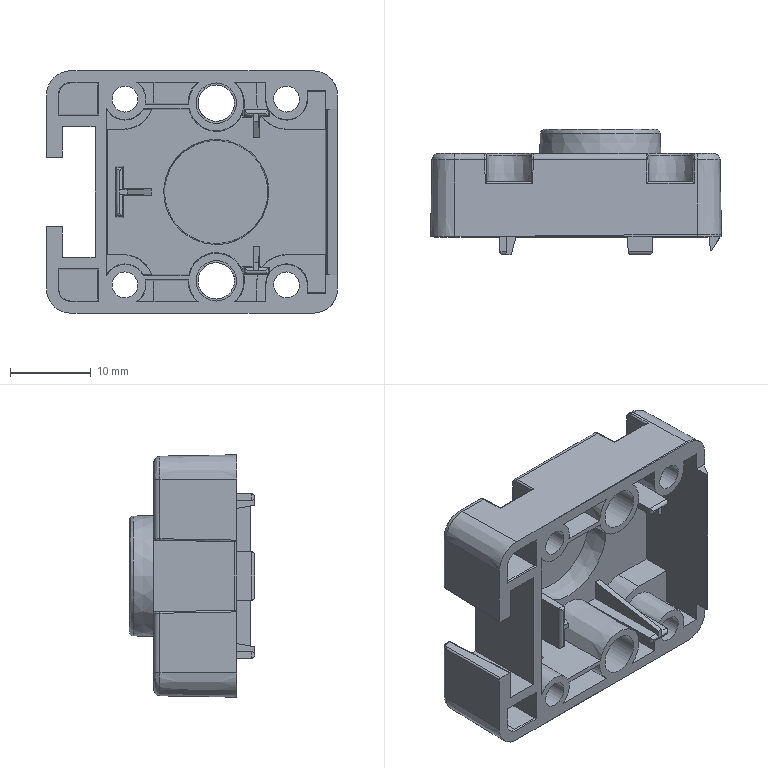Part | NX | 1 solid | 234 faces | box 36.005 x 15.5 x 30.01 mm | volume 4180 mm3 | plane 123 | cylinder 62 | cone 30 | spline 19 | commonest cylinder face diameters 0.4 x26 0.8 x15 1.6 x9 3.2 x4 3.14 x2 4.5 x2